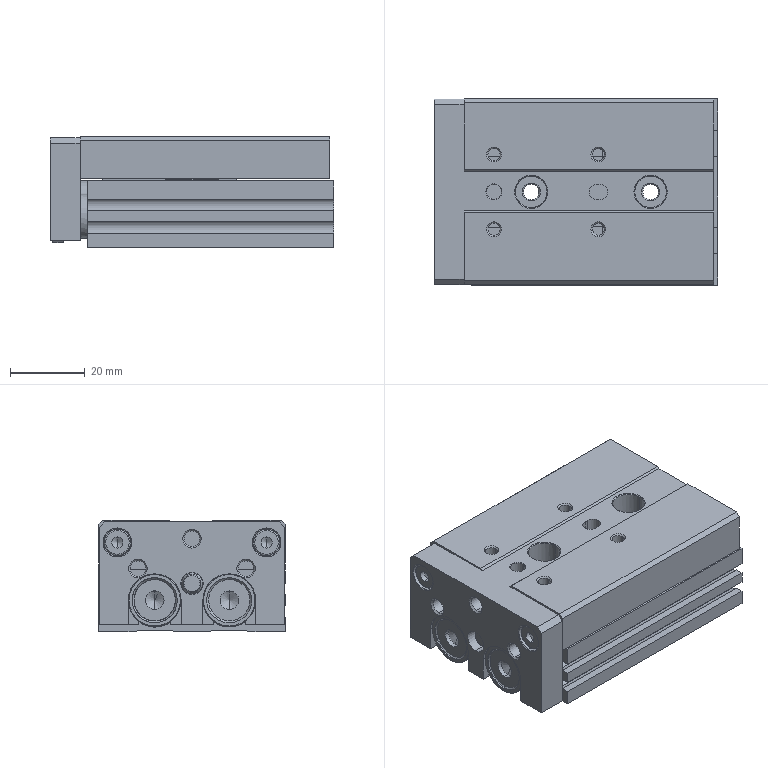Part | SolidWorks | 2 solids | 430 faces | box 76 x 50 x 30 mm | volume 87070 mm3 | plane 176 | cylinder 158 | cone 90 | spline 6 | commonest cylinder face diameters 3.242 x24 4.134 x14 12 x12 4 x10 6 x10 7.5 x8